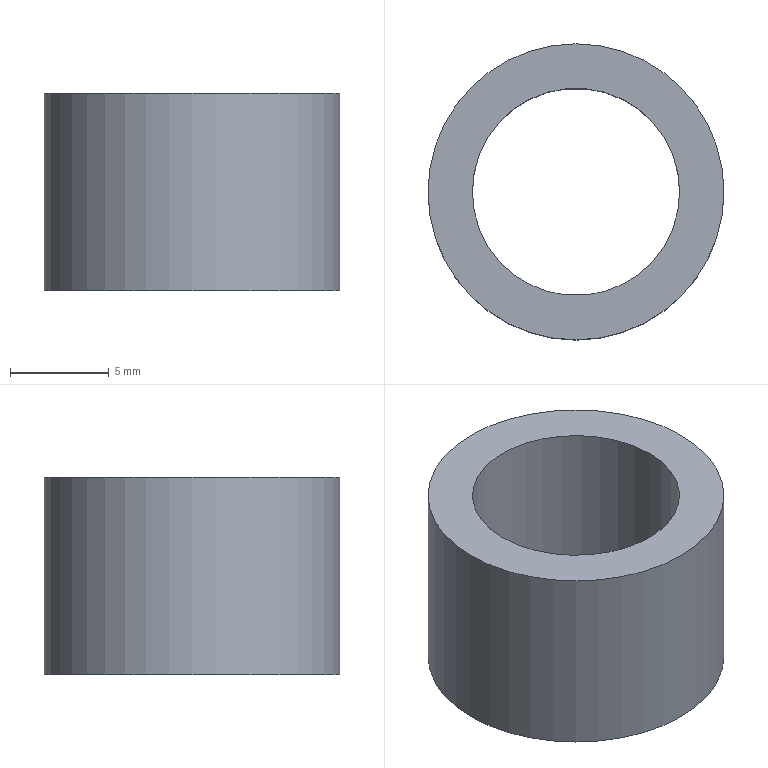Part | NX | features DATUM_CSYS 1, EXTRACT_DATUM_PLANE 1, EXTRUDE 1, SKETCH 1 | 1 solid | 4 faces | box 15 x 15 x 10 mm | volume 901.244 mm3 | cylinder 2 | plane 2 | commonest cylinder face diameters 10.5 x1 15 x1
STEP:
#1=CARTESIAN_POINT('',(7.5,0.,0.));
#2=VERTEX_POINT('',#1);
#3=CARTESIAN_POINT('',(0.,0.,0.));
#4=DIRECTION('',(0.,0.,1.));
#5=DIRECTION('',(1.,0.,0.));
#6=AXIS2_PLACEMENT_3D('',#3,#4,#5);
#7=CIRCLE('',#6,7.5);
#8=EDGE_CURVE('',#2,#2,#7,.T.);
#9=ORIENTED_EDGE('',*,*,#8,.T.);
#10=EDGE_LOOP('',(#9));
#11=FACE_BOUND('',#10,.T.);
#12=CARTESIAN_POINT('',(7.5,0.,10.));
#13=VERTEX_POINT('',#12);
#14=CARTESIAN_POINT('',(0.,0.,10.));
#15=DIRECTION('',(0.,0.,1.));
#16=DIRECTION('',(1.,0.,0.));
#17=AXIS2_PLACEMENT_3D('',#14,#15,#16);
#18=CIRCLE('',#17,7.5);
#19=EDGE_CURVE('',#13,#13,#18,.T.);
#20=ORIENTED_EDGE('',*,*,#19,.F.);
#21=EDGE_LOOP('',(#20));
#22=FACE_BOUND('',#21,.T.);
#23=CARTESIAN_POINT('',(0.,0.,0.));
#24=DIRECTION('',(0.,0.,1.));
#25=DIRECTION('',(1.,0.,0.));
#26=AXIS2_PLACEMENT_3D('',#23,#24,#25);
#27=CYLINDRICAL_SURFACE('',#26,7.5);
#28=ADVANCED_FACE('',(#11,#22),#27,.T.);
#29=CARTESIAN_POINT('',(5.25,0.,0.));
#30=VERTEX_POINT('',#29);
#31=CARTESIAN_POINT('',(0.,0.,0.));
#32=DIRECTION('',(0.,0.,1.));
#33=DIRECTION('',(1.,0.,0.));
#34=AXIS2_PLACEMENT_3D('',#31,#32,#33);
#35=CIRCLE('',#34,5.25);
#36=EDGE_CURVE('',#30,#30,#35,.T.);
#37=ORIENTED_EDGE('',*,*,#36,.F.);
#38=EDGE_LOOP('',(#37));
#39=FACE_BOUND('',#38,.T.);
#40=CARTESIAN_POINT('',(5.25,0.,10.));
#41=VERTEX_POINT('',#40);
#42=CARTESIAN_POINT('',(0.,0.,10.));
#43=DIRECTION('',(0.,0.,1.));
#44=DIRECTION('',(1.,0.,0.));
#45=AXIS2_PLACEMENT_3D('',#42,#43,#44);
#46=CIRCLE('',#45,5.25);
#47=EDGE_CURVE('',#41,#41,#46,.T.);
#48=ORIENTED_EDGE('',*,*,#47,.T.);
#49=EDGE_LOOP('',(#48));
#50=FACE_BOUND('',#49,.T.);
#51=CARTESIAN_POINT('',(0.,0.,0.));
#52=DIRECTION('',(0.,0.,1.));
#53=DIRECTION('',(1.,0.,0.));
#54=AXIS2_PLACEMENT_3D('',#51,#52,#53);
#55=CYLINDRICAL_SURFACE('',#54,5.25);
#56=ADVANCED_FACE('',(#39,#50),#55,.F.);
#57=ORIENTED_EDGE('',*,*,#8,.F.);
#58=EDGE_LOOP('',(#57));
#59=FACE_BOUND('',#58,.T.);
#60=ORIENTED_EDGE('',*,*,#36,.T.);
#61=EDGE_LOOP('',(#60));
#62=FACE_BOUND('',#61,.T.);
#63=CARTESIAN_POINT('',(0.,0.,0.));
#64=DIRECTION('',(0.,0.,1.));
#65=DIRECTION('',(1.,0.,0.));
#66=AXIS2_PLACEMENT_3D('',#63,#64,#65);
#67=PLANE('',#66);
#68=ADVANCED_FACE('',(#59,#62),#67,.F.);
#69=ORIENTED_EDGE('',*,*,#19,.T.);
#70=EDGE_LOOP('',(#69));
#71=FACE_BOUND('',#70,.T.);
#72=ORIENTED_EDGE('',*,*,#47,.F.);
#73=EDGE_LOOP('',(#72));
#74=FACE_BOUND('',#73,.T.);
#75=CARTESIAN_POINT('',(0.,0.,10.));
#76=DIRECTION('',(0.,0.,1.));
#77=DIRECTION('',(1.,0.,0.));
#78=AXIS2_PLACEMENT_3D('',#75,#76,#77);
#79=PLANE('',#78);
#80=ADVANCED_FACE('',(#71,#74),#79,.T.);
#81=CLOSED_SHELL('',(#28,#56,#68,#80));
#82=MANIFOLD_SOLID_BREP('',#81);
#83=(LENGTH_UNIT()NAMED_UNIT(*)SI_UNIT(.MILLI.,.METRE.));
#84=UNCERTAINTY_MEASURE_WITH_UNIT(LENGTH_MEASURE(0.00001),#83,'','');
#85=(NAMED_UNIT(*)PLANE_ANGLE_UNIT()SI_UNIT($,.RADIAN.));
#86=(NAMED_UNIT(*)SI_UNIT($,.STERADIAN.)SOLID_ANGLE_UNIT());
#87=(GEOMETRIC_REPRESENTATION_CONTEXT(3)GLOBAL_UNCERTAINTY_ASSIGNED_CONTEXT((#84))GLOBAL_UNIT_ASSIGNED_CONTEXT((#83,#85,#86))REPRESENTATION_CONTEXT('',''));
#88=ADVANCED_BREP_SHAPE_REPRESENTATION('',(#82),#87);